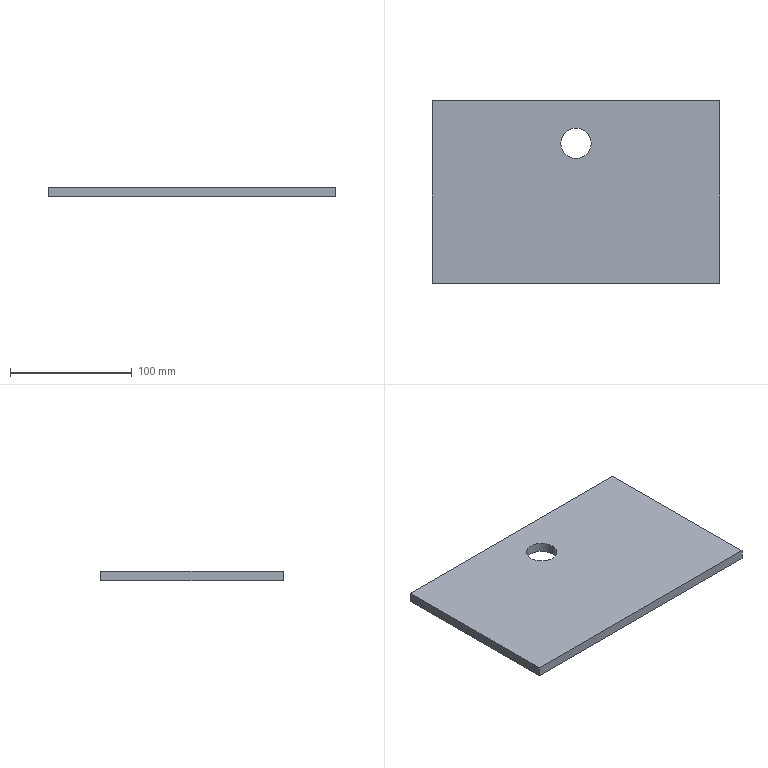Part | SolidWorks | features Extrusion 1, HoleWzd 1 | 1 solid | 8 faces | box 236 x 150 x 8 mm | volume 279273 mm3 | plane 6 | cylinder 2 | commonest cylinder face diameters 25 x2
STEP:
#1=CARTESIAN_POINT('',(-12.5,40.,-4.));
#2=VERTEX_POINT('',#1);
#3=CARTESIAN_POINT('',(12.5,40.,-4.));
#4=VERTEX_POINT('',#3);
#5=CARTESIAN_POINT('',(0.,40.,-4.));
#6=DIRECTION('',(0.,0.,1.));
#7=DIRECTION('',(1.,0.,0.));
#8=AXIS2_PLACEMENT_3D('',#5,#6,#7);
#9=CIRCLE('',#8,12.5);
#10=EDGE_CURVE('',#2,#4,#9,.T.);
#11=ORIENTED_EDGE('',*,*,#10,.F.);
#12=CARTESIAN_POINT('',(-12.5,40.,4.));
#13=VERTEX_POINT('',#12);
#14=CARTESIAN_POINT('',(-12.5,40.,4.));
#15=DIRECTION('',(0.,0.,1.));
#16=VECTOR('',#15,1000.);
#17=LINE('',#14,#16);
#18=EDGE_CURVE('',#2,#13,#17,.T.);
#19=ORIENTED_EDGE('',*,*,#18,.T.);
#20=CARTESIAN_POINT('',(12.5,40.,4.));
#21=VERTEX_POINT('',#20);
#22=CARTESIAN_POINT('',(0.,40.,4.));
#23=DIRECTION('',(0.,0.,1.));
#24=DIRECTION('',(1.,0.,0.));
#25=AXIS2_PLACEMENT_3D('',#22,#23,#24);
#26=CIRCLE('',#25,12.5);
#27=EDGE_CURVE('',#13,#21,#26,.T.);
#28=ORIENTED_EDGE('',*,*,#27,.T.);
#29=CARTESIAN_POINT('',(12.5,40.,4.));
#30=DIRECTION('',(0.,0.,1.));
#31=VECTOR('',#30,1000.);
#32=LINE('',#29,#31);
#33=EDGE_CURVE('',#4,#21,#32,.T.);
#34=ORIENTED_EDGE('',*,*,#33,.F.);
#35=EDGE_LOOP('',(#11,#19,#28,#34));
#36=FACE_OUTER_BOUND('',#35,.T.);
#37=CARTESIAN_POINT('',(0.,40.,4.));
#38=DIRECTION('',(0.,0.,1.));
#39=DIRECTION('',(1.,0.,0.));
#40=AXIS2_PLACEMENT_3D('',#37,#38,#39);
#41=CYLINDRICAL_SURFACE('',#40,12.5);
#42=ADVANCED_FACE('',(#36),#41,.F.);
#43=CARTESIAN_POINT('',(-118.,75.,-4.));
#44=VERTEX_POINT('',#43);
#45=CARTESIAN_POINT('',(-118.,-75.,-4.));
#46=VERTEX_POINT('',#45);
#47=CARTESIAN_POINT('',(-118.,-75.,-4.));
#48=DIRECTION('',(0.,-1.,0.));
#49=VECTOR('',#48,1000.);
#50=LINE('',#47,#49);
#51=EDGE_CURVE('',#44,#46,#50,.T.);
#52=ORIENTED_EDGE('',*,*,#51,.T.);
#53=CARTESIAN_POINT('',(-118.,-75.,4.));
#54=VERTEX_POINT('',#53);
#55=CARTESIAN_POINT('',(-118.,-75.,4.));
#56=DIRECTION('',(0.,0.,-1.));
#57=VECTOR('',#56,1000.);
#58=LINE('',#55,#57);
#59=EDGE_CURVE('',#54,#46,#58,.T.);
#60=ORIENTED_EDGE('',*,*,#59,.F.);
#61=CARTESIAN_POINT('',(-118.,75.,4.));
#62=VERTEX_POINT('',#61);
#63=CARTESIAN_POINT('',(-118.,-75.,4.));
#64=DIRECTION('',(0.,-1.,0.));
#65=VECTOR('',#64,1000.);
#66=LINE('',#63,#65);
#67=EDGE_CURVE('',#62,#54,#66,.T.);
#68=ORIENTED_EDGE('',*,*,#67,.F.);
#69=CARTESIAN_POINT('',(-118.,75.,4.));
#70=DIRECTION('',(0.,0.,-1.));
#71=VECTOR('',#70,1000.);
#72=LINE('',#69,#71);
#73=EDGE_CURVE('',#62,#44,#72,.T.);
#74=ORIENTED_EDGE('',*,*,#73,.T.);
#75=EDGE_LOOP('',(#52,#60,#68,#74));
#76=FACE_OUTER_BOUND('',#75,.T.);
#77=CARTESIAN_POINT('',(-118.,-75.,4.));
#78=DIRECTION('',(1.,0.,0.));
#79=DIRECTION('',(0.,0.,-1.));
#80=AXIS2_PLACEMENT_3D('',#77,#78,#79);
#81=PLANE('',#80);
#82=ADVANCED_FACE('',(#76),#81,.F.);
#83=CARTESIAN_POINT('',(118.,-75.,-4.));
#84=VERTEX_POINT('',#83);
#85=CARTESIAN_POINT('',(118.,-75.,-4.));
#86=DIRECTION('',(1.,0.,0.));
#87=VECTOR('',#86,1000.);
#88=LINE('',#85,#87);
#89=EDGE_CURVE('',#46,#84,#88,.T.);
#90=ORIENTED_EDGE('',*,*,#89,.T.);
#91=CARTESIAN_POINT('',(118.,-75.,4.));
#92=VERTEX_POINT('',#91);
#93=CARTESIAN_POINT('',(118.,-75.,4.));
#94=DIRECTION('',(0.,0.,-1.));
#95=VECTOR('',#94,1000.);
#96=LINE('',#93,#95);
#97=EDGE_CURVE('',#92,#84,#96,.T.);
#98=ORIENTED_EDGE('',*,*,#97,.F.);
#99=CARTESIAN_POINT('',(118.,-75.,4.));
#100=DIRECTION('',(1.,0.,0.));
#101=VECTOR('',#100,1000.);
#102=LINE('',#99,#101);
#103=EDGE_CURVE('',#54,#92,#102,.T.);
#104=ORIENTED_EDGE('',*,*,#103,.F.);
#105=ORIENTED_EDGE('',*,*,#59,.T.);
#106=EDGE_LOOP('',(#90,#98,#104,#105));
#107=FACE_OUTER_BOUND('',#106,.T.);
#108=CARTESIAN_POINT('',(118.,-75.,4.));
#109=DIRECTION('',(0.,1.,0.));
#110=DIRECTION('',(-1.,0.,0.));
#111=AXIS2_PLACEMENT_3D('',#108,#109,#110);
#112=PLANE('',#111);
#113=ADVANCED_FACE('',(#107),#112,.F.);
#114=CARTESIAN_POINT('',(118.,75.,-4.));
#115=VERTEX_POINT('',#114);
#116=CARTESIAN_POINT('',(118.,-75.,-4.));
#117=DIRECTION('',(0.,1.,0.));
#118=VECTOR('',#117,1000.);
#119=LINE('',#116,#118);
#120=EDGE_CURVE('',#84,#115,#119,.T.);
#121=ORIENTED_EDGE('',*,*,#120,.T.);
#122=CARTESIAN_POINT('',(118.,75.,4.));
#123=VERTEX_POINT('',#122);
#124=CARTESIAN_POINT('',(118.,75.,4.));
#125=DIRECTION('',(0.,0.,-1.));
#126=VECTOR('',#125,1000.);
#127=LINE('',#124,#126);
#128=EDGE_CURVE('',#123,#115,#127,.T.);
#129=ORIENTED_EDGE('',*,*,#128,.F.);
#130=CARTESIAN_POINT('',(118.,-75.,4.));
#131=DIRECTION('',(0.,1.,0.));
#132=VECTOR('',#131,1000.);
#133=LINE('',#130,#132);
#134=EDGE_CURVE('',#92,#123,#133,.T.);
#135=ORIENTED_EDGE('',*,*,#134,.F.);
#136=ORIENTED_EDGE('',*,*,#97,.T.);
#137=EDGE_LOOP('',(#121,#129,#135,#136));
#138=FACE_OUTER_BOUND('',#137,.T.);
#139=CARTESIAN_POINT('',(118.,-75.,4.));
#140=DIRECTION('',(-1.,0.,0.));
#141=DIRECTION('',(0.,0.,1.));
#142=AXIS2_PLACEMENT_3D('',#139,#140,#141);
#143=PLANE('',#142);
#144=ADVANCED_FACE('',(#138),#143,.F.);
#145=CARTESIAN_POINT('',(118.,75.,-4.));
#146=DIRECTION('',(-1.,0.,0.));
#147=VECTOR('',#146,1000.);
#148=LINE('',#145,#147);
#149=EDGE_CURVE('',#115,#44,#148,.T.);
#150=ORIENTED_EDGE('',*,*,#149,.T.);
#151=ORIENTED_EDGE('',*,*,#73,.F.);
#152=CARTESIAN_POINT('',(118.,75.,4.));
#153=DIRECTION('',(-1.,0.,0.));
#154=VECTOR('',#153,1000.);
#155=LINE('',#152,#154);
#156=EDGE_CURVE('',#123,#62,#155,.T.);
#157=ORIENTED_EDGE('',*,*,#156,.F.);
#158=ORIENTED_EDGE('',*,*,#128,.T.);
#159=EDGE_LOOP('',(#150,#151,#157,#158));
#160=FACE_OUTER_BOUND('',#159,.T.);
#161=CARTESIAN_POINT('',(118.,75.,4.));
#162=DIRECTION('',(0.,-1.,0.));
#163=DIRECTION('',(1.,0.,0.));
#164=AXIS2_PLACEMENT_3D('',#161,#162,#163);
#165=PLANE('',#164);
#166=ADVANCED_FACE('',(#160),#165,.F.);
#167=CARTESIAN_POINT('',(0.,40.,4.));
#168=DIRECTION('',(0.,0.,1.));
#169=DIRECTION('',(1.,0.,0.));
#170=AXIS2_PLACEMENT_3D('',#167,#168,#169);
#171=CIRCLE('',#170,12.5);
#172=EDGE_CURVE('',#21,#13,#171,.T.);
#173=ORIENTED_EDGE('',*,*,#172,.F.);
#174=ORIENTED_EDGE('',*,*,#27,.F.);
#175=EDGE_LOOP('',(#173,#174));
#176=FACE_BOUND('',#175,.T.);
#177=ORIENTED_EDGE('',*,*,#67,.T.);
#178=ORIENTED_EDGE('',*,*,#103,.T.);
#179=ORIENTED_EDGE('',*,*,#134,.T.);
#180=ORIENTED_EDGE('',*,*,#156,.T.);
#181=EDGE_LOOP('',(#177,#178,#179,#180));
#182=FACE_OUTER_BOUND('',#181,.T.);
#183=CARTESIAN_POINT('',(0.,0.,4.));
#184=DIRECTION('',(0.,0.,1.));
#185=DIRECTION('',(1.,0.,0.));
#186=AXIS2_PLACEMENT_3D('',#183,#184,#185);
#187=PLANE('',#186);
#188=ADVANCED_FACE('',(#176,#182),#187,.T.);
#189=CARTESIAN_POINT('',(0.,40.,-4.));
#190=DIRECTION('',(0.,0.,1.));
#191=DIRECTION('',(1.,0.,0.));
#192=AXIS2_PLACEMENT_3D('',#189,#190,#191);
#193=CIRCLE('',#192,12.5);
#194=EDGE_CURVE('',#4,#2,#193,.T.);
#195=ORIENTED_EDGE('',*,*,#194,.T.);
#196=ORIENTED_EDGE('',*,*,#10,.T.);
#197=EDGE_LOOP('',(#195,#196));
#198=FACE_BOUND('',#197,.T.);
#199=ORIENTED_EDGE('',*,*,#51,.F.);
#200=ORIENTED_EDGE('',*,*,#149,.F.);
#201=ORIENTED_EDGE('',*,*,#120,.F.);
#202=ORIENTED_EDGE('',*,*,#89,.F.);
#203=EDGE_LOOP('',(#199,#200,#201,#202));
#204=FACE_OUTER_BOUND('',#203,.T.);
#205=CARTESIAN_POINT('',(0.,0.,-4.));
#206=DIRECTION('',(0.,0.,1.));
#207=DIRECTION('',(1.,0.,0.));
#208=AXIS2_PLACEMENT_3D('',#205,#206,#207);
#209=PLANE('',#208);
#210=ADVANCED_FACE('',(#198,#204),#209,.F.);
#211=ORIENTED_EDGE('',*,*,#18,.F.);
#212=ORIENTED_EDGE('',*,*,#194,.F.);
#213=ORIENTED_EDGE('',*,*,#33,.T.);
#214=ORIENTED_EDGE('',*,*,#172,.T.);
#215=EDGE_LOOP('',(#211,#212,#213,#214));
#216=FACE_OUTER_BOUND('',#215,.T.);
#217=CARTESIAN_POINT('',(0.,40.,4.));
#218=DIRECTION('',(0.,0.,1.));
#219=DIRECTION('',(1.,0.,0.));
#220=AXIS2_PLACEMENT_3D('',#217,#218,#219);
#221=CYLINDRICAL_SURFACE('',#220,12.5);
#222=ADVANCED_FACE('',(#216),#221,.F.);
#223=CLOSED_SHELL('',(#42,#82,#113,#144,#166,#188,#210,#222));
#224=MANIFOLD_SOLID_BREP('',#223);
#225=CARTESIAN_POINT('',(0.,0.,0.));
#226=DIRECTION('',(0.,0.,1.));
#227=DIRECTION('',(1.,0.,0.));
#228=AXIS2_PLACEMENT_3D('',#225,#226,#227);
#229=(LENGTH_UNIT()NAMED_UNIT(*)SI_UNIT(.MILLI.,.METRE.));
#230=UNCERTAINTY_MEASURE_WITH_UNIT(LENGTH_MEASURE(0.00001),#229,'','');
#231=(NAMED_UNIT(*)PLANE_ANGLE_UNIT()SI_UNIT($,.RADIAN.));
#232=(NAMED_UNIT(*)SI_UNIT($,.STERADIAN.)SOLID_ANGLE_UNIT());
#233=(GEOMETRIC_REPRESENTATION_CONTEXT(3)GLOBAL_UNCERTAINTY_ASSIGNED_CONTEXT((#230))GLOBAL_UNIT_ASSIGNED_CONTEXT((#229,#231,#232))REPRESENTATION_CONTEXT('',''));
#234=ADVANCED_BREP_SHAPE_REPRESENTATION('',(#224,#228),#233);